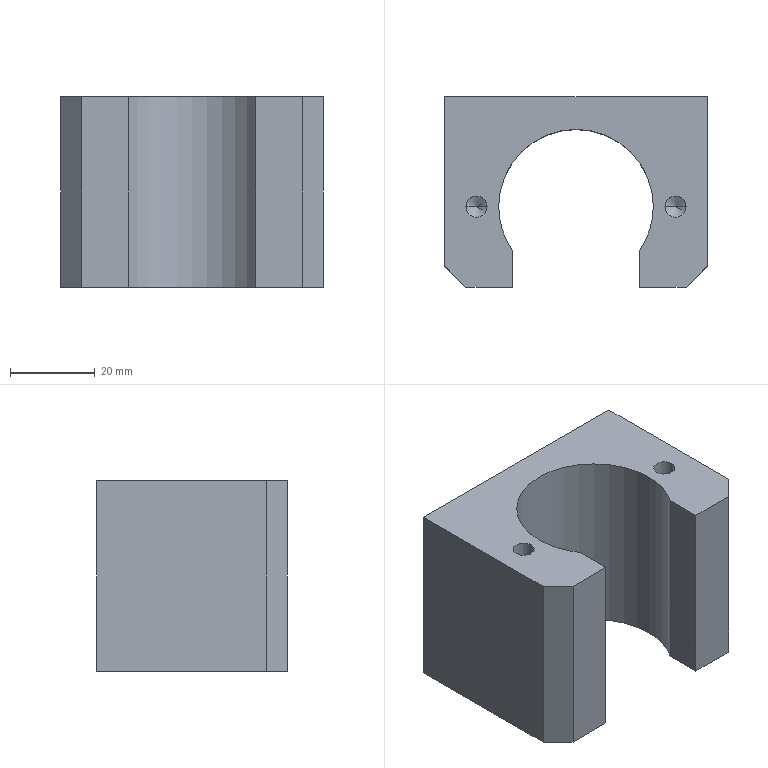Part | SolidWorks | features HoleWzd 2, Chamfer 1, Extrusion 1, ICE 1, MirrorPattern 1 | 1 solid | 46 faces | box 62 x 45 x 45 mm | volume 70731 mm3 | cylinder 19 | cone 16 | plane 11 | commonest cylinder face diameters 5 x16 36.5 x3
STEP:
#1=CARTESIAN_POINT('',(21.,-3.5,7.5));
#2=VERTEX_POINT('',#1);
#3=CARTESIAN_POINT('',(26.,-3.5,7.5));
#4=VERTEX_POINT('',#3);
#5=CARTESIAN_POINT('',(23.5,-3.5,7.5));
#6=DIRECTION('',(0.,0.,1.));
#7=DIRECTION('',(1.,0.,0.));
#8=AXIS2_PLACEMENT_3D('',#5,#6,#7);
#9=CIRCLE('',#8,2.5);
#10=EDGE_CURVE('',#2,#4,#9,.T.);
#11=ORIENTED_EDGE('',*,*,#10,.F.);
#12=CARTESIAN_POINT('',(21.,-3.5,22.5));
#13=VERTEX_POINT('',#12);
#14=CARTESIAN_POINT('',(21.,-3.5,22.5));
#15=DIRECTION('',(0.,0.,1.));
#16=VECTOR('',#15,1000.);
#17=LINE('',#14,#16);
#18=EDGE_CURVE('',#2,#13,#17,.T.);
#19=ORIENTED_EDGE('',*,*,#18,.T.);
#20=CARTESIAN_POINT('',(26.,-3.5,22.5));
#21=VERTEX_POINT('',#20);
#22=CARTESIAN_POINT('',(23.5,-3.5,22.5));
#23=DIRECTION('',(0.,0.,1.));
#24=DIRECTION('',(1.,0.,0.));
#25=AXIS2_PLACEMENT_3D('',#22,#23,#24);
#26=CIRCLE('',#25,2.5);
#27=EDGE_CURVE('',#13,#21,#26,.T.);
#28=ORIENTED_EDGE('',*,*,#27,.T.);
#29=CARTESIAN_POINT('',(26.,-3.5,22.5));
#30=DIRECTION('',(0.,0.,1.));
#31=VECTOR('',#30,1000.);
#32=LINE('',#29,#31);
#33=EDGE_CURVE('',#4,#21,#32,.T.);
#34=ORIENTED_EDGE('',*,*,#33,.F.);
#35=EDGE_LOOP('',(#11,#19,#28,#34));
#36=FACE_OUTER_BOUND('',#35,.T.);
#37=CARTESIAN_POINT('',(23.5,-3.5,22.5));
#38=DIRECTION('',(0.,0.,1.));
#39=DIRECTION('',(1.,0.,0.));
#40=AXIS2_PLACEMENT_3D('',#37,#38,#39);
#41=CYLINDRICAL_SURFACE('',#40,2.5);
#42=ADVANCED_FACE('',(#36),#41,.F.);
#43=CARTESIAN_POINT('',(23.5,-3.5,5.998));
#44=VERTEX_POINT('',#43);
#45=CARTESIAN_POINT('',(26.,-3.5,7.5));
#46=DIRECTION('',(0.8572,0.,0.515));
#47=VECTOR('',#46,1000.);
#48=LINE('',#45,#47);
#49=EDGE_CURVE('',#44,#4,#48,.T.);
#50=ORIENTED_EDGE('',*,*,#49,.F.);
#51=CARTESIAN_POINT('',(21.,-3.5,7.5));
#52=DIRECTION('',(-0.8572,0.,0.515));
#53=VECTOR('',#52,1000.);
#54=LINE('',#51,#53);
#55=EDGE_CURVE('',#44,#2,#54,.T.);
#56=ORIENTED_EDGE('',*,*,#55,.T.);
#57=ORIENTED_EDGE('',*,*,#10,.T.);
#58=EDGE_LOOP('',(#50,#56,#57));
#59=FACE_OUTER_BOUND('',#58,.T.);
#60=CARTESIAN_POINT('',(23.5,-3.5,7.5));
#61=DIRECTION('',(0.,0.,1.));
#62=DIRECTION('',(1.,0.,0.));
#63=AXIS2_PLACEMENT_3D('',#60,#61,#62);
#64=CONICAL_SURFACE('',#63,2.5,1.03);
#65=ADVANCED_FACE('',(#59),#64,.F.);
#66=CARTESIAN_POINT('',(-26.,-3.5,7.5));
#67=VERTEX_POINT('',#66);
#68=CARTESIAN_POINT('',(-21.,-3.5,7.5));
#69=VERTEX_POINT('',#68);
#70=CARTESIAN_POINT('',(-23.5,-3.5,7.5));
#71=DIRECTION('',(0.,0.,1.));
#72=DIRECTION('',(1.,0.,0.));
#73=AXIS2_PLACEMENT_3D('',#70,#71,#72);
#74=CIRCLE('',#73,2.5);
#75=EDGE_CURVE('',#67,#69,#74,.T.);
#76=ORIENTED_EDGE('',*,*,#75,.F.);
#77=CARTESIAN_POINT('',(-26.,-3.5,22.5));
#78=VERTEX_POINT('',#77);
#79=CARTESIAN_POINT('',(-26.,-3.5,22.5));
#80=DIRECTION('',(0.,0.,1.));
#81=VECTOR('',#80,1000.);
#82=LINE('',#79,#81);
#83=EDGE_CURVE('',#67,#78,#82,.T.);
#84=ORIENTED_EDGE('',*,*,#83,.T.);
#85=CARTESIAN_POINT('',(-21.,-3.5,22.5));
#86=VERTEX_POINT('',#85);
#87=CARTESIAN_POINT('',(-23.5,-3.5,22.5));
#88=DIRECTION('',(0.,0.,1.));
#89=DIRECTION('',(1.,0.,0.));
#90=AXIS2_PLACEMENT_3D('',#87,#88,#89);
#91=CIRCLE('',#90,2.5);
#92=EDGE_CURVE('',#78,#86,#91,.T.);
#93=ORIENTED_EDGE('',*,*,#92,.T.);
#94=CARTESIAN_POINT('',(-21.,-3.5,22.5));
#95=DIRECTION('',(0.,0.,1.));
#96=VECTOR('',#95,1000.);
#97=LINE('',#94,#96);
#98=EDGE_CURVE('',#69,#86,#97,.T.);
#99=ORIENTED_EDGE('',*,*,#98,.F.);
#100=EDGE_LOOP('',(#76,#84,#93,#99));
#101=FACE_OUTER_BOUND('',#100,.T.);
#102=CARTESIAN_POINT('',(-23.5,-3.5,22.5));
#103=DIRECTION('',(0.,0.,1.));
#104=DIRECTION('',(1.,0.,0.));
#105=AXIS2_PLACEMENT_3D('',#102,#103,#104);
#106=CYLINDRICAL_SURFACE('',#105,2.5);
#107=ADVANCED_FACE('',(#101),#106,.F.);
#108=CARTESIAN_POINT('',(-23.5,-3.5,5.998));
#109=VERTEX_POINT('',#108);
#110=CARTESIAN_POINT('',(-21.,-3.5,7.5));
#111=DIRECTION('',(0.8572,0.,0.515));
#112=VECTOR('',#111,1000.);
#113=LINE('',#110,#112);
#114=EDGE_CURVE('',#109,#69,#113,.T.);
#115=ORIENTED_EDGE('',*,*,#114,.F.);
#116=CARTESIAN_POINT('',(-26.,-3.5,7.5));
#117=DIRECTION('',(-0.8572,0.,0.515));
#118=VECTOR('',#117,1000.);
#119=LINE('',#116,#118);
#120=EDGE_CURVE('',#109,#67,#119,.T.);
#121=ORIENTED_EDGE('',*,*,#120,.T.);
#122=ORIENTED_EDGE('',*,*,#75,.T.);
#123=EDGE_LOOP('',(#115,#121,#122));
#124=FACE_OUTER_BOUND('',#123,.T.);
#125=CARTESIAN_POINT('',(-23.5,-3.5,7.5));
#126=DIRECTION('',(0.,0.,1.));
#127=DIRECTION('',(1.,0.,0.));
#128=AXIS2_PLACEMENT_3D('',#125,#126,#127);
#129=CONICAL_SURFACE('',#128,2.5,1.03);
#130=ADVANCED_FACE('',(#124),#129,.F.);
#131=CARTESIAN_POINT('',(26.,-3.5,-7.5));
#132=VERTEX_POINT('',#131);
#133=CARTESIAN_POINT('',(21.,-3.5,-7.5));
#134=VERTEX_POINT('',#133);
#135=CARTESIAN_POINT('',(23.5,-3.5,-7.5));
#136=DIRECTION('',(0.,0.,-1.));
#137=DIRECTION('',(-1.,0.,0.));
#138=AXIS2_PLACEMENT_3D('',#135,#136,#137);
#139=CIRCLE('',#138,2.5);
#140=EDGE_CURVE('',#132,#134,#139,.T.);
#141=ORIENTED_EDGE('',*,*,#140,.F.);
#142=CARTESIAN_POINT('',(26.,-3.5,-22.5));
#143=VERTEX_POINT('',#142);
#144=CARTESIAN_POINT('',(26.,-3.5,-22.5));
#145=DIRECTION('',(0.,0.,-1.));
#146=VECTOR('',#145,1000.);
#147=LINE('',#144,#146);
#148=EDGE_CURVE('',#132,#143,#147,.T.);
#149=ORIENTED_EDGE('',*,*,#148,.T.);
#150=CARTESIAN_POINT('',(21.,-3.5,-22.5));
#151=VERTEX_POINT('',#150);
#152=CARTESIAN_POINT('',(23.5,-3.5,-22.5));
#153=DIRECTION('',(0.,0.,-1.));
#154=DIRECTION('',(-1.,0.,0.));
#155=AXIS2_PLACEMENT_3D('',#152,#153,#154);
#156=CIRCLE('',#155,2.5);
#157=EDGE_CURVE('',#143,#151,#156,.T.);
#158=ORIENTED_EDGE('',*,*,#157,.T.);
#159=CARTESIAN_POINT('',(21.,-3.5,-22.5));
#160=DIRECTION('',(0.,0.,-1.));
#161=VECTOR('',#160,1000.);
#162=LINE('',#159,#161);
#163=EDGE_CURVE('',#134,#151,#162,.T.);
#164=ORIENTED_EDGE('',*,*,#163,.F.);
#165=EDGE_LOOP('',(#141,#149,#158,#164));
#166=FACE_OUTER_BOUND('',#165,.T.);
#167=CARTESIAN_POINT('',(23.5,-3.5,-22.5));
#168=DIRECTION('',(0.,0.,-1.));
#169=DIRECTION('',(-1.,0.,0.));
#170=AXIS2_PLACEMENT_3D('',#167,#168,#169);
#171=CYLINDRICAL_SURFACE('',#170,2.5);
#172=ADVANCED_FACE('',(#166),#171,.F.);
#173=CARTESIAN_POINT('',(23.5,-3.5,-5.998));
#174=VERTEX_POINT('',#173);
#175=CARTESIAN_POINT('',(21.,-3.5,-7.5));
#176=DIRECTION('',(-0.8572,0.,-0.515));
#177=VECTOR('',#176,1000.);
#178=LINE('',#175,#177);
#179=EDGE_CURVE('',#174,#134,#178,.T.);
#180=ORIENTED_EDGE('',*,*,#179,.F.);
#181=CARTESIAN_POINT('',(26.,-3.5,-7.5));
#182=DIRECTION('',(0.8572,0.,-0.515));
#183=VECTOR('',#182,1000.);
#184=LINE('',#181,#183);
#185=EDGE_CURVE('',#174,#132,#184,.T.);
#186=ORIENTED_EDGE('',*,*,#185,.T.);
#187=ORIENTED_EDGE('',*,*,#140,.T.);
#188=EDGE_LOOP('',(#180,#186,#187));
#189=FACE_OUTER_BOUND('',#188,.T.);
#190=CARTESIAN_POINT('',(23.5,-3.5,-7.5));
#191=DIRECTION('',(0.,0.,-1.));
#192=DIRECTION('',(-1.,0.,0.));
#193=AXIS2_PLACEMENT_3D('',#190,#191,#192);
#194=CONICAL_SURFACE('',#193,2.5,1.03);
#195=ADVANCED_FACE('',(#189),#194,.F.);
#196=CARTESIAN_POINT('',(-21.,-3.5,-7.5));
#197=VERTEX_POINT('',#196);
#198=CARTESIAN_POINT('',(-26.,-3.5,-7.5));
#199=VERTEX_POINT('',#198);
#200=CARTESIAN_POINT('',(-23.5,-3.5,-7.5));
#201=DIRECTION('',(0.,0.,-1.));
#202=DIRECTION('',(-1.,0.,0.));
#203=AXIS2_PLACEMENT_3D('',#200,#201,#202);
#204=CIRCLE('',#203,2.5);
#205=EDGE_CURVE('',#197,#199,#204,.T.);
#206=ORIENTED_EDGE('',*,*,#205,.F.);
#207=CARTESIAN_POINT('',(-21.,-3.5,-22.5));
#208=VERTEX_POINT('',#207);
#209=CARTESIAN_POINT('',(-21.,-3.5,-22.5));
#210=DIRECTION('',(0.,0.,-1.));
#211=VECTOR('',#210,1000.);
#212=LINE('',#209,#211);
#213=EDGE_CURVE('',#197,#208,#212,.T.);
#214=ORIENTED_EDGE('',*,*,#213,.T.);
#215=CARTESIAN_POINT('',(-26.,-3.5,-22.5));
#216=VERTEX_POINT('',#215);
#217=CARTESIAN_POINT('',(-23.5,-3.5,-22.5));
#218=DIRECTION('',(0.,0.,-1.));
#219=DIRECTION('',(-1.,0.,0.));
#220=AXIS2_PLACEMENT_3D('',#217,#218,#219);
#221=CIRCLE('',#220,2.5);
#222=EDGE_CURVE('',#208,#216,#221,.T.);
#223=ORIENTED_EDGE('',*,*,#222,.T.);
#224=CARTESIAN_POINT('',(-26.,-3.5,-22.5));
#225=DIRECTION('',(0.,0.,-1.));
#226=VECTOR('',#225,1000.);
#227=LINE('',#224,#226);
#228=EDGE_CURVE('',#199,#216,#227,.T.);
#229=ORIENTED_EDGE('',*,*,#228,.F.);
#230=EDGE_LOOP('',(#206,#214,#223,#229));
#231=FACE_OUTER_BOUND('',#230,.T.);
#232=CARTESIAN_POINT('',(-23.5,-3.5,-22.5));
#233=DIRECTION('',(0.,0.,-1.));
#234=DIRECTION('',(-1.,0.,0.));
#235=AXIS2_PLACEMENT_3D('',#232,#233,#234);
#236=CYLINDRICAL_SURFACE('',#235,2.5);
#237=ADVANCED_FACE('',(#231),#236,.F.);
#238=CARTESIAN_POINT('',(-23.5,-3.5,-5.998));
#239=VERTEX_POINT('',#238);
#240=CARTESIAN_POINT('',(-26.,-3.5,-7.5));
#241=DIRECTION('',(-0.8572,0.,-0.515));
#242=VECTOR('',#241,1000.);
#243=LINE('',#240,#242);
#244=EDGE_CURVE('',#239,#199,#243,.T.);
#245=ORIENTED_EDGE('',*,*,#244,.F.);
#246=CARTESIAN_POINT('',(-21.,-3.5,-7.5));
#247=DIRECTION('',(0.8572,0.,-0.515));
#248=VECTOR('',#247,1000.);
#249=LINE('',#246,#248);
#250=EDGE_CURVE('',#239,#197,#249,.T.);
#251=ORIENTED_EDGE('',*,*,#250,.T.);
#252=ORIENTED_EDGE('',*,*,#205,.T.);
#253=EDGE_LOOP('',(#245,#251,#252));
#254=FACE_OUTER_BOUND('',#253,.T.);
#255=CARTESIAN_POINT('',(-23.5,-3.5,-7.5));
#256=DIRECTION('',(0.,0.,-1.));
#257=DIRECTION('',(-1.,0.,0.));
#258=AXIS2_PLACEMENT_3D('',#255,#256,#257);
#259=CONICAL_SURFACE('',#258,2.5,1.03);
#260=ADVANCED_FACE('',(#254),#259,.F.);
#261=CARTESIAN_POINT('',(-25.,7.5,-17.5));
#262=VERTEX_POINT('',#261);
#263=CARTESIAN_POINT('',(-25.,7.5,-12.5));
#264=VERTEX_POINT('',#263);
#265=CARTESIAN_POINT('',(-25.,7.5,-15.));
#266=DIRECTION('',(0.,1.,0.));
#267=DIRECTION('',(0.,0.,1.));
#268=AXIS2_PLACEMENT_3D('',#265,#266,#267);
#269=CIRCLE('',#268,2.5);
#270=EDGE_CURVE('',#262,#264,#269,.T.);
#271=ORIENTED_EDGE('',*,*,#270,.F.);
#272=CARTESIAN_POINT('',(-25.,22.5,-17.5));
#273=VERTEX_POINT('',#272);
#274=CARTESIAN_POINT('',(-25.,22.5,-17.5));
#275=DIRECTION('',(0.,1.,0.));
#276=VECTOR('',#275,1000.);
#277=LINE('',#274,#276);
#278=EDGE_CURVE('',#262,#273,#277,.T.);
#279=ORIENTED_EDGE('',*,*,#278,.T.);
#280=CARTESIAN_POINT('',(-25.,22.5,-12.5));
#281=VERTEX_POINT('',#280);
#282=CARTESIAN_POINT('',(-25.,22.5,-15.));
#283=DIRECTION('',(0.,1.,0.));
#284=DIRECTION('',(0.,0.,1.));
#285=AXIS2_PLACEMENT_3D('',#282,#283,#284);
#286=CIRCLE('',#285,2.5);
#287=EDGE_CURVE('',#273,#281,#286,.T.);
#288=ORIENTED_EDGE('',*,*,#287,.T.);
#289=CARTESIAN_POINT('',(-25.,22.5,-12.5));
#290=DIRECTION('',(0.,1.,0.));
#291=VECTOR('',#290,1000.);
#292=LINE('',#289,#291);
#293=EDGE_CURVE('',#264,#281,#292,.T.);
#294=ORIENTED_EDGE('',*,*,#293,.F.);
#295=EDGE_LOOP('',(#271,#279,#288,#294));
#296=FACE_OUTER_BOUND('',#295,.T.);
#297=CARTESIAN_POINT('',(-25.,22.5,-15.));
#298=DIRECTION('',(0.,1.,0.));
#299=DIRECTION('',(0.,0.,1.));
#300=AXIS2_PLACEMENT_3D('',#297,#298,#299);
#301=CYLINDRICAL_SURFACE('',#300,2.5);
#302=ADVANCED_FACE('',(#296),#301,.F.);
#303=CARTESIAN_POINT('',(-25.,5.998,-15.));
#304=VERTEX_POINT('',#303);
#305=CARTESIAN_POINT('',(-25.,7.5,-12.5));
#306=DIRECTION('',(0.,0.515,0.8572));
#307=VECTOR('',#306,1000.);
#308=LINE('',#305,#307);
#309=EDGE_CURVE('',#304,#264,#308,.T.);
#310=ORIENTED_EDGE('',*,*,#309,.F.);
#311=CARTESIAN_POINT('',(-25.,7.5,-17.5));
#312=DIRECTION('',(0.,0.515,-0.8572));
#313=VECTOR('',#312,1000.);
#314=LINE('',#311,#313);
#315=EDGE_CURVE('',#304,#262,#314,.T.);
#316=ORIENTED_EDGE('',*,*,#315,.T.);
#317=ORIENTED_EDGE('',*,*,#270,.T.);
#318=EDGE_LOOP('',(#310,#316,#317));
#319=FACE_OUTER_BOUND('',#318,.T.);
#320=CARTESIAN_POINT('',(-25.,7.5,-15.));
#321=DIRECTION('',(0.,1.,0.));
#322=DIRECTION('',(0.,0.,1.));
#323=AXIS2_PLACEMENT_3D('',#320,#321,#322);
#324=CONICAL_SURFACE('',#323,2.5,1.03);
#325=ADVANCED_FACE('',(#319),#324,.F.);
#326=CARTESIAN_POINT('',(-25.,7.5,12.5));
#327=VERTEX_POINT('',#326);
#328=CARTESIAN_POINT('',(-25.,7.5,17.5));
#329=VERTEX_POINT('',#328);
#330=CARTESIAN_POINT('',(-25.,7.5,15.));
#331=DIRECTION('',(0.,1.,0.));
#332=DIRECTION('',(0.,0.,1.));
#333=AXIS2_PLACEMENT_3D('',#330,#331,#332);
#334=CIRCLE('',#333,2.5);
#335=EDGE_CURVE('',#327,#329,#334,.T.);
#336=ORIENTED_EDGE('',*,*,#335,.F.);
#337=CARTESIAN_POINT('',(-25.,22.5,12.5));
#338=VERTEX_POINT('',#337);
#339=CARTESIAN_POINT('',(-25.,22.5,12.5));
#340=DIRECTION('',(0.,1.,0.));
#341=VECTOR('',#340,1000.);
#342=LINE('',#339,#341);
#343=EDGE_CURVE('',#327,#338,#342,.T.);
#344=ORIENTED_EDGE('',*,*,#343,.T.);
#345=CARTESIAN_POINT('',(-25.,22.5,17.5));
#346=VERTEX_POINT('',#345);
#347=CARTESIAN_POINT('',(-25.,22.5,15.));
#348=DIRECTION('',(0.,1.,0.));
#349=DIRECTION('',(0.,0.,1.));
#350=AXIS2_PLACEMENT_3D('',#347,#348,#349);
#351=CIRCLE('',#350,2.5);
#352=EDGE_CURVE('',#338,#346,#351,.T.);
#353=ORIENTED_EDGE('',*,*,#352,.T.);
#354=CARTESIAN_POINT('',(-25.,22.5,17.5));
#355=DIRECTION('',(0.,1.,0.));
#356=VECTOR('',#355,1000.);
#357=LINE('',#354,#356);
#358=EDGE_CURVE('',#329,#346,#357,.T.);
#359=ORIENTED_EDGE('',*,*,#358,.F.);
#360=EDGE_LOOP('',(#336,#344,#353,#359));
#361=FACE_OUTER_BOUND('',#360,.T.);
#362=CARTESIAN_POINT('',(-25.,22.5,15.));
#363=DIRECTION('',(0.,1.,0.));
#364=DIRECTION('',(0.,0.,1.));
#365=AXIS2_PLACEMENT_3D('',#362,#363,#364);
#366=CYLINDRICAL_SURFACE('',#365,2.5);
#367=ADVANCED_FACE('',(#361),#366,.F.);
#368=CARTESIAN_POINT('',(-25.,5.998,15.));
#369=VERTEX_POINT('',#368);
#370=CARTESIAN_POINT('',(-25.,7.5,17.5));
#371=DIRECTION('',(0.,0.515,0.8572));
#372=VECTOR('',#371,1000.);
#373=LINE('',#370,#372);
#374=EDGE_CURVE('',#369,#329,#373,.T.);
#375=ORIENTED_EDGE('',*,*,#374,.F.);
#376=CARTESIAN_POINT('',(-25.,7.5,12.5));
#377=DIRECTION('',(0.,0.515,-0.8572));
#378=VECTOR('',#377,1000.);
#379=LINE('',#376,#378);
#380=EDGE_CURVE('',#369,#327,#379,.T.);
#381=ORIENTED_EDGE('',*,*,#380,.T.);
#382=ORIENTED_EDGE('',*,*,#335,.T.);
#383=EDGE_LOOP('',(#375,#381,#382));
#384=FACE_OUTER_BOUND('',#383,.T.);
#385=CARTESIAN_POINT('',(-25.,7.5,15.));
#386=DIRECTION('',(0.,1.,0.));
#387=DIRECTION('',(0.,0.,1.));
#388=AXIS2_PLACEMENT_3D('',#385,#386,#387);
#389=CONICAL_SURFACE('',#388,2.5,1.03);
#390=ADVANCED_FACE('',(#384),#389,.F.);
#391=CARTESIAN_POINT('',(25.,7.5,12.5));
#392=VERTEX_POINT('',#391);
#393=CARTESIAN_POINT('',(25.,7.5,17.5));
#394=VERTEX_POINT('',#393);
#395=CARTESIAN_POINT('',(25.,7.5,15.));
#396=DIRECTION('',(0.,1.,0.));
#397=DIRECTION('',(0.,0.,1.));
#398=AXIS2_PLACEMENT_3D('',#395,#396,#397);
#399=CIRCLE('',#398,2.5);
#400=EDGE_CURVE('',#392,#394,#399,.T.);
#401=ORIENTED_EDGE('',*,*,#400,.F.);
#402=CARTESIAN_POINT('',(25.,22.5,12.5));
#403=VERTEX_POINT('',#402);
#404=CARTESIAN_POINT('',(25.,22.5,12.5));
#405=DIRECTION('',(0.,1.,0.));
#406=VECTOR('',#405,1000.);
#407=LINE('',#404,#406);
#408=EDGE_CURVE('',#392,#403,#407,.T.);
#409=ORIENTED_EDGE('',*,*,#408,.T.);
#410=CARTESIAN_POINT('',(25.,22.5,17.5));
#411=VERTEX_POINT('',#410);
#412=CARTESIAN_POINT('',(25.,22.5,15.));
#413=DIRECTION('',(0.,1.,0.));
#414=DIRECTION('',(0.,0.,1.));
#415=AXIS2_PLACEMENT_3D('',#412,#413,#414);
#416=CIRCLE('',#415,2.5);
#417=EDGE_CURVE('',#403,#411,#416,.T.);
#418=ORIENTED_EDGE('',*,*,#417,.T.);
#419=CARTESIAN_POINT('',(25.,22.5,17.5));
#420=DIRECTION('',(0.,1.,0.));
#421=VECTOR('',#420,1000.);
#422=LINE('',#419,#421);
#423=EDGE_CURVE('',#394,#411,#422,.T.);
#424=ORIENTED_EDGE('',*,*,#423,.F.);
#425=EDGE_LOOP('',(#401,#409,#418,#424));
#426=FACE_OUTER_BOUND('',#425,.T.);
#427=CARTESIAN_POINT('',(25.,22.5,15.));
#428=DIRECTION('',(0.,1.,0.));
#429=DIRECTION('',(0.,0.,1.));
#430=AXIS2_PLACEMENT_3D('',#427,#428,#429);
#431=CYLINDRICAL_SURFACE('',#430,2.5);
#432=ADVANCED_FACE('',(#426),#431,.F.);
#433=CARTESIAN_POINT('',(25.,5.998,15.));
#434=VERTEX_POINT('',#433);
#435=CARTESIAN_POINT('',(25.,7.5,17.5));
#436=DIRECTION('',(0.,0.515,0.8572));
#437=VECTOR('',#436,1000.);
#438=LINE('',#435,#437);
#439=EDGE_CURVE('',#434,#394,#438,.T.);
#440=ORIENTED_EDGE('',*,*,#439,.F.);
#441=CARTESIAN_POINT('',(25.,7.5,12.5));
#442=DIRECTION('',(0.,0.515,-0.8572));
#443=VECTOR('',#442,1000.);
#444=LINE('',#441,#443);
#445=EDGE_CURVE('',#434,#392,#444,.T.);
#446=ORIENTED_EDGE('',*,*,#445,.T.);
#447=ORIENTED_EDGE('',*,*,#400,.T.);
#448=EDGE_LOOP('',(#440,#446,#447));
#449=FACE_OUTER_BOUND('',#448,.T.);
#450=CARTESIAN_POINT('',(25.,7.5,15.));
#451=DIRECTION('',(0.,1.,0.));
#452=DIRECTION('',(0.,0.,1.));
#453=AXIS2_PLACEMENT_3D('',#450,#451,#452);
#454=CONICAL_SURFACE('',#453,2.5,1.03);
#455=ADVANCED_FACE('',(#449),#454,.F.);
#456=CARTESIAN_POINT('',(25.,7.5,-17.5));
#457=VERTEX_POINT('',#456);
#458=CARTESIAN_POINT('',(25.,7.5,-12.5));
#459=VERTEX_POINT('',#458);
#460=CARTESIAN_POINT('',(25.,7.5,-15.));
#461=DIRECTION('',(0.,1.,0.));
#462=DIRECTION('',(0.,0.,1.));
#463=AXIS2_PLACEMENT_3D('',#460,#461,#462);
#464=CIRCLE('',#463,2.5);
#465=EDGE_CURVE('',#457,#459,#464,.T.);
#466=ORIENTED_EDGE('',*,*,#465,.F.);
#467=CARTESIAN_POINT('',(25.,22.5,-17.5));
#468=VERTEX_POINT('',#467);
#469=CARTESIAN_POINT('',(25.,22.5,-17.5));
#470=DIRECTION('',(0.,1.,0.));
#471=VECTOR('',#470,1000.);
#472=LINE('',#469,#471);
#473=EDGE_CURVE('',#457,#468,#472,.T.);
#474=ORIENTED_EDGE('',*,*,#473,.T.);
#475=CARTESIAN_POINT('',(25.,22.5,-12.5));
#476=VERTEX_POINT('',#475);
#477=CARTESIAN_POINT('',(25.,22.5,-15.));
#478=DIRECTION('',(0.,1.,0.));
#479=DIRECTION('',(0.,0.,1.));
#480=AXIS2_PLACEMENT_3D('',#477,#478,#479);
#481=CIRCLE('',#480,2.5);
#482=EDGE_CURVE('',#468,#476,#481,.T.);
#483=ORIENTED_EDGE('',*,*,#482,.T.);
#484=CARTESIAN_POINT('',(25.,22.5,-12.5));
#485=DIRECTION('',(0.,1.,0.));
#486=VECTOR('',#485,1000.);
#487=LINE('',#484,#486);
#488=EDGE_CURVE('',#459,#476,#487,.T.);
#489=ORIENTED_EDGE('',*,*,#488,.F.);
#490=EDGE_LOOP('',(#466,#474,#483,#489));
#491=FACE_OUTER_BOUND('',#490,.T.);
#492=CARTESIAN_POINT('',(25.,22.5,-15.));
#493=DIRECTION('',(0.,1.,0.));
#494=DIRECTION('',(0.,0.,1.));
#495=AXIS2_PLACEMENT_3D('',#492,#493,#494);
#496=CYLINDRICAL_SURFACE('',#495,2.5);
#497=ADVANCED_FACE('',(#491),#496,.F.);
#498=CARTESIAN_POINT('',(25.,5.998,-15.));
#499=VERTEX_POINT('',#498);
#500=CARTESIAN_POINT('',(25.,7.5,-12.5));
#501=DIRECTION('',(0.,0.515,0.8572));
#502=VECTOR('',#501,1000.);
#503=LINE('',#500,#502);
#504=EDGE_CURVE('',#499,#459,#503,.T.);
#505=ORIENTED_EDGE('',*,*,#504,.F.);
#506=CARTESIAN_POINT('',(25.,7.5,-17.5));
#507=DIRECTION('',(0.,0.515,-0.8572));
#508=VECTOR('',#507,1000.);
#509=LINE('',#506,#508);
#510=EDGE_CURVE('',#499,#457,#509,.T.);
#511=ORIENTED_EDGE('',*,*,#510,.T.);
#512=ORIENTED_EDGE('',*,*,#465,.T.);
#513=EDGE_LOOP('',(#505,#511,#512));
#514=FACE_OUTER_BOUND('',#513,.T.);
#515=CARTESIAN_POINT('',(25.,7.5,-15.));
#516=DIRECTION('',(0.,1.,0.));
#517=DIRECTION('',(0.,0.,1.));
#518=AXIS2_PLACEMENT_3D('',#515,#516,#517);
#519=CONICAL_SURFACE('',#518,2.5,1.03);
#520=ADVANCED_FACE('',(#514),#519,.F.);
#521=CARTESIAN_POINT('',(15.,-13.895,22.5));
#522=VERTEX_POINT('',#521);
#523=CARTESIAN_POINT('',(18.25,-3.5,22.5));
#524=VERTEX_POINT('',#523);
#525=CARTESIAN_POINT('',(0.,-3.5,22.5));
#526=DIRECTION('',(0.,0.,1.));
#527=DIRECTION('',(-1.,0.,0.));
#528=AXIS2_PLACEMENT_3D('',#525,#526,#527);
#529=CIRCLE('',#528,18.25);
#530=EDGE_CURVE('',#522,#524,#529,.T.);
#531=ORIENTED_EDGE('',*,*,#530,.T.);
#532=CARTESIAN_POINT('',(18.25,-3.5,-22.5));
#533=VERTEX_POINT('',#532);
#534=CARTESIAN_POINT('',(18.25,-3.5,74.652));
#535=DIRECTION('',(0.,0.,-1.));
#536=VECTOR('',#535,1000.);
#537=LINE('',#534,#536);
#538=EDGE_CURVE('',#524,#533,#537,.T.);
#539=ORIENTED_EDGE('',*,*,#538,.T.);
#540=CARTESIAN_POINT('',(15.,-13.895,-22.5));
#541=VERTEX_POINT('',#540);
#542=CARTESIAN_POINT('',(0.,-3.5,-22.5));
#543=DIRECTION('',(0.,0.,-1.));
#544=DIRECTION('',(-1.,0.,0.));
#545=AXIS2_PLACEMENT_3D('',#542,#543,#544);
#546=CIRCLE('',#545,18.25);
#547=EDGE_CURVE('',#533,#541,#546,.T.);
#548=ORIENTED_EDGE('',*,*,#547,.T.);
#549=CARTESIAN_POINT('',(15.,-13.895,74.652));
#550=DIRECTION('',(0.,0.,-1.));
#551=VECTOR('',#550,1000.);
#552=LINE('',#549,#551);
#553=EDGE_CURVE('',#522,#541,#552,.T.);
#554=ORIENTED_EDGE('',*,*,#553,.F.);
#555=EDGE_LOOP('',(#531,#539,#548,#554));
#556=FACE_OUTER_BOUND('',#555,.T.);
#557=CARTESIAN_POINT('',(0.,-3.5,74.652));
#558=DIRECTION('',(0.,0.,-1.));
#559=DIRECTION('',(-1.,0.,0.));
#560=AXIS2_PLACEMENT_3D('',#557,#558,#559);
#561=CYLINDRICAL_SURFACE('',#560,18.25);
#562=ADVANCED_FACE('',(#556),#561,.F.);
#563=ORIENTED_EDGE('',*,*,#538,.F.);
#564=CARTESIAN_POINT('',(-18.25,-3.5,22.5));
#565=VERTEX_POINT('',#564);
#566=CARTESIAN_POINT('',(0.,-3.5,22.5));
#567=DIRECTION('',(0.,0.,1.));
#568=DIRECTION('',(-1.,0.,0.));
#569=AXIS2_PLACEMENT_3D('',#566,#567,#568);
#570=CIRCLE('',#569,18.25);
#571=EDGE_CURVE('',#524,#565,#570,.T.);
#572=ORIENTED_EDGE('',*,*,#571,.T.);
#573=CARTESIAN_POINT('',(-18.25,-3.5,-22.5));
#574=VERTEX_POINT('',#573);
#575=CARTESIAN_POINT('',(-18.25,-3.5,74.652));
#576=DIRECTION('',(0.,0.,-1.));
#577=VECTOR('',#576,1000.);
#578=LINE('',#575,#577);
#579=EDGE_CURVE('',#565,#574,#578,.T.);
#580=ORIENTED_EDGE('',*,*,#579,.T.);
#581=CARTESIAN_POINT('',(0.,-3.5,-22.5));
#582=DIRECTION('',(0.,0.,-1.));
#583=DIRECTION('',(-1.,0.,0.));
#584=AXIS2_PLACEMENT_3D('',#581,#582,#583);
#585=CIRCLE('',#584,18.25);
#586=EDGE_CURVE('',#574,#533,#585,.T.);
#587=ORIENTED_EDGE('',*,*,#586,.T.);
#588=EDGE_LOOP('',(#563,#572,#580,#587));
#589=FACE_OUTER_BOUND('',#588,.T.);
#590=CARTESIAN_POINT('',(0.,-3.5,74.652));
#591=DIRECTION('',(0.,0.,-1.));
#592=DIRECTION('',(-1.,0.,0.));
#593=AXIS2_PLACEMENT_3D('',#590,#591,#592);
#594=CYLINDRICAL_SURFACE('',#593,18.25);
#595=ADVANCED_FACE('',(#589),#594,.F.);
#596=CARTESIAN_POINT('',(-26.,-22.5,22.5));
#597=VERTEX_POINT('',#596);
#598=CARTESIAN_POINT('',(-15.,-22.5,22.5));
#599=VERTEX_POINT('',#598);
#600=CARTESIAN_POINT('',(-31.,-22.5,22.5));
#601=DIRECTION('',(1.,0.,0.));
#602=VECTOR('',#601,1000.);
#603=LINE('',#600,#602);
#604=EDGE_CURVE('',#597,#599,#603,.T.);
#605=ORIENTED_EDGE('',*,*,#604,.F.);
#606=CARTESIAN_POINT('',(-26.,-22.5,-22.5));
#607=VERTEX_POINT('',#606);
#608=CARTESIAN_POINT('',(-26.,-22.5,-22.5));
#609=DIRECTION('',(0.,0.,-1.));
#610=VECTOR('',#609,1000.);
#611=LINE('',#608,#610);
#612=EDGE_CURVE('',#597,#607,#611,.T.);
#613=ORIENTED_EDGE('',*,*,#612,.T.);
#614=CARTESIAN_POINT('',(-15.,-22.5,-22.5));
#615=VERTEX_POINT('',#614);
#616=CARTESIAN_POINT('',(-31.,-22.5,-22.5));
#617=DIRECTION('',(-1.,0.,0.));
#618=VECTOR('',#617,1000.);
#619=LINE('',#616,#618);
#620=EDGE_CURVE('',#615,#607,#619,.T.);
#621=ORIENTED_EDGE('',*,*,#620,.F.);
#622=CARTESIAN_POINT('',(-15.,-22.5,74.652));
#623=DIRECTION('',(0.,0.,-1.));
#624=VECTOR('',#623,1000.);
#625=LINE('',#622,#624);
#626=EDGE_CURVE('',#599,#615,#625,.T.);
#627=ORIENTED_EDGE('',*,*,#626,.F.);
#628=EDGE_LOOP('',(#605,#613,#621,#627));
#629=FACE_OUTER_BOUND('',#628,.T.);
#630=CARTESIAN_POINT('',(0.,-22.5,0.));
#631=DIRECTION('',(0.,-1.,0.));
#632=DIRECTION('',(0.,0.,-1.));
#633=AXIS2_PLACEMENT_3D('',#630,#631,#632);
#634=PLANE('',#633);
#635=ADVANCED_FACE('',(#629),#634,.T.);
#636=CARTESIAN_POINT('',(31.,22.5,22.5));
#637=VERTEX_POINT('',#636);
#638=CARTESIAN_POINT('',(31.,-17.5,22.5));
#639=VERTEX_POINT('',#638);
#640=CARTESIAN_POINT('',(31.,22.5,22.5));
#641=DIRECTION('',(0.,-1.,0.));
#642=VECTOR('',#641,1000.);
#643=LINE('',#640,#642);
#644=EDGE_CURVE('',#637,#639,#643,.T.);
#645=ORIENTED_EDGE('',*,*,#644,.T.);
#646=CARTESIAN_POINT('',(31.,-17.5,-22.5));
#647=VERTEX_POINT('',#646);
#648=CARTESIAN_POINT('',(31.,-17.5,-22.5));
#649=DIRECTION('',(0.,0.,-1.));
#650=VECTOR('',#649,1000.);
#651=LINE('',#648,#650);
#652=EDGE_CURVE('',#639,#647,#651,.T.);
#653=ORIENTED_EDGE('',*,*,#652,.T.);
#654=CARTESIAN_POINT('',(31.,22.5,-22.5));
#655=VERTEX_POINT('',#654);
#656=CARTESIAN_POINT('',(31.,22.5,-22.5));
#657=DIRECTION('',(0.,-1.,0.));
#658=VECTOR('',#657,1000.);
#659=LINE('',#656,#658);
#660=EDGE_CURVE('',#655,#647,#659,.T.);
#661=ORIENTED_EDGE('',*,*,#660,.F.);
#662=CARTESIAN_POINT('',(31.,22.5,22.5));
#663=DIRECTION('',(0.,0.,-1.));
#664=VECTOR('',#663,1000.);
#665=LINE('',#662,#664);
#666=EDGE_CURVE('',#637,#655,#665,.T.);
#667=ORIENTED_EDGE('',*,*,#666,.F.);
#668=EDGE_LOOP('',(#645,#653,#661,#667));
#669=FACE_OUTER_BOUND('',#668,.T.);
#670=CARTESIAN_POINT('',(31.,22.5,22.5));
#671=DIRECTION('',(-1.,0.,0.));
#672=DIRECTION('',(0.,0.,1.));
#673=AXIS2_PLACEMENT_3D('',#670,#671,#672);
#674=PLANE('',#673);
#675=ADVANCED_FACE('',(#669),#674,.F.);
#676=CARTESIAN_POINT('',(23.5,-3.5,-22.5));
#677=DIRECTION('',(0.,0.,-1.));
#678=DIRECTION('',(-1.,0.,0.));
#679=AXIS2_PLACEMENT_3D('',#676,#677,#678);
#680=CIRCLE('',#679,2.5);
#681=EDGE_CURVE('',#151,#143,#680,.T.);
#682=ORIENTED_EDGE('',*,*,#681,.F.);
#683=ORIENTED_EDGE('',*,*,#157,.F.);
#684=EDGE_LOOP('',(#682,#683));
#685=FACE_BOUND('',#684,.T.);
#686=CARTESIAN_POINT('',(-23.5,-3.5,-22.5));
#687=DIRECTION('',(0.,0.,-1.));
#688=DIRECTION('',(-1.,0.,0.));
#689=AXIS2_PLACEMENT_3D('',#686,#687,#688);
#690=CIRCLE('',#689,2.5);
#691=EDGE_CURVE('',#216,#208,#690,.T.);
#692=ORIENTED_EDGE('',*,*,#691,.F.);
#693=ORIENTED_EDGE('',*,*,#222,.F.);
#694=EDGE_LOOP('',(#692,#693));
#695=FACE_BOUND('',#694,.T.);
#696=ORIENTED_EDGE('',*,*,#660,.T.);
#697=CARTESIAN_POINT('',(26.,-22.5,-22.5));
#698=VERTEX_POINT('',#697);
#699=CARTESIAN_POINT('',(31.,-17.5,-22.5));
#700=DIRECTION('',(-0.7071,-0.7071,0.));
#701=VECTOR('',#700,1000.);
#702=LINE('',#699,#701);
#703=EDGE_CURVE('',#647,#698,#702,.T.);
#704=ORIENTED_EDGE('',*,*,#703,.T.);
#705=CARTESIAN_POINT('',(15.,-22.5,-22.5));
#706=VERTEX_POINT('',#705);
#707=CARTESIAN_POINT('',(-31.,-22.5,-22.5));
#708=DIRECTION('',(-1.,0.,0.));
#709=VECTOR('',#708,1000.);
#710=LINE('',#707,#709);
#711=EDGE_CURVE('',#698,#706,#710,.T.);
#712=ORIENTED_EDGE('',*,*,#711,.T.);
#713=CARTESIAN_POINT('',(15.,-13.895,-22.5));
#714=DIRECTION('',(0.,-1.,0.));
#715=VECTOR('',#714,1000.);
#716=LINE('',#713,#715);
#717=EDGE_CURVE('',#541,#706,#716,.T.);
#718=ORIENTED_EDGE('',*,*,#717,.F.);
#719=ORIENTED_EDGE('',*,*,#547,.F.);
#720=ORIENTED_EDGE('',*,*,#586,.F.);
#721=CARTESIAN_POINT('',(-15.,-13.895,-22.5));
#722=VERTEX_POINT('',#721);
#723=CARTESIAN_POINT('',(0.,-3.5,-22.5));
#724=DIRECTION('',(0.,0.,-1.));
#725=DIRECTION('',(-1.,0.,0.));
#726=AXIS2_PLACEMENT_3D('',#723,#724,#725);
#727=CIRCLE('',#726,18.25);
#728=EDGE_CURVE('',#722,#574,#727,.T.);
#729=ORIENTED_EDGE('',*,*,#728,.F.);
#730=CARTESIAN_POINT('',(-15.,-13.895,-22.5));
#731=DIRECTION('',(0.,1.,0.));
#732=VECTOR('',#731,1000.);
#733=LINE('',#730,#732);
#734=EDGE_CURVE('',#615,#722,#733,.T.);
#735=ORIENTED_EDGE('',*,*,#734,.F.);
#736=ORIENTED_EDGE('',*,*,#620,.T.);
#737=CARTESIAN_POINT('',(-31.,-17.5,-22.5));
#738=VERTEX_POINT('',#737);
#739=CARTESIAN_POINT('',(-31.,-17.5,-22.5));
#740=DIRECTION('',(-0.7071,0.7071,0.));
#741=VECTOR('',#740,1000.);
#742=LINE('',#739,#741);
#743=EDGE_CURVE('',#607,#738,#742,.T.);
#744=ORIENTED_EDGE('',*,*,#743,.T.);
#745=CARTESIAN_POINT('',(-31.,22.5,-22.5));
#746=VERTEX_POINT('',#745);
#747=CARTESIAN_POINT('',(-31.,22.5,-22.5));
#748=DIRECTION('',(0.,-1.,0.));
#749=VECTOR('',#748,1000.);
#750=LINE('',#747,#749);
#751=EDGE_CURVE('',#746,#738,#750,.T.);
#752=ORIENTED_EDGE('',*,*,#751,.F.);
#753=CARTESIAN_POINT('',(-31.,22.5,-22.5));
#754=DIRECTION('',(-1.,0.,0.));
#755=VECTOR('',#754,1000.);
#756=LINE('',#753,#755);
#757=EDGE_CURVE('',#655,#746,#756,.T.);
#758=ORIENTED_EDGE('',*,*,#757,.F.);
#759=EDGE_LOOP('',(#696,#704,#712,#718,#719,#720,#729,#735,#736,#744,#752,#758));
#760=FACE_OUTER_BOUND('',#759,.T.);
#761=CARTESIAN_POINT('',(-31.,22.5,-22.5));
#762=DIRECTION('',(0.,0.,1.));
#763=DIRECTION('',(1.,0.,0.));
#764=AXIS2_PLACEMENT_3D('',#761,#762,#763);
#765=PLANE('',#764);
#766=ADVANCED_FACE('',(#685,#695,#760),#765,.F.);
#767=ORIENTED_EDGE('',*,*,#751,.T.);
#768=CARTESIAN_POINT('',(-31.,-17.5,22.5));
#769=VERTEX_POINT('',#768);
#770=CARTESIAN_POINT('',(-31.,-17.5,22.5));
#771=DIRECTION('',(0.,0.,1.));
#772=VECTOR('',#771,1000.);
#773=LINE('',#770,#772);
#774=EDGE_CURVE('',#738,#769,#773,.T.);
#775=ORIENTED_EDGE('',*,*,#774,.T.);
#776=CARTESIAN_POINT('',(-31.,22.5,22.5));
#777=VERTEX_POINT('',#776);
#778=CARTESIAN_POINT('',(-31.,22.5,22.5));
#779=DIRECTION('',(0.,-1.,0.));
#780=VECTOR('',#779,1000.);
#781=LINE('',#778,#780);
#782=EDGE_CURVE('',#777,#769,#781,.T.);
#783=ORIENTED_EDGE('',*,*,#782,.F.);
#784=CARTESIAN_POINT('',(-31.,22.5,22.5));
#785=DIRECTION('',(0.,0.,1.));
#786=VECTOR('',#785,1000.);
#787=LINE('',#784,#786);
#788=EDGE_CURVE('',#746,#777,#787,.T.);
#789=ORIENTED_EDGE('',*,*,#788,.F.);
#790=EDGE_LOOP('',(#767,#775,#783,#789));
#791=FACE_OUTER_BOUND('',#790,.T.);
#792=CARTESIAN_POINT('',(-31.,22.5,22.5));
#793=DIRECTION('',(1.,0.,0.));
#794=DIRECTION('',(0.,0.,-1.));
#795=AXIS2_PLACEMENT_3D('',#792,#793,#794);
#796=PLANE('',#795);
#797=ADVANCED_FACE('',(#791),#796,.F.);
#798=CARTESIAN_POINT('',(23.5,-3.5,22.5));
#799=DIRECTION('',(0.,0.,1.));
#800=DIRECTION('',(1.,0.,0.));
#801=AXIS2_PLACEMENT_3D('',#798,#799,#800);
#802=CIRCLE('',#801,2.5);
#803=EDGE_CURVE('',#21,#13,#802,.T.);
#804=ORIENTED_EDGE('',*,*,#803,.F.);
#805=ORIENTED_EDGE('',*,*,#27,.F.);
#806=EDGE_LOOP('',(#804,#805));
#807=FACE_BOUND('',#806,.T.);
#808=CARTESIAN_POINT('',(-23.5,-3.5,22.5));
#809=DIRECTION('',(0.,0.,1.));
#810=DIRECTION('',(1.,0.,0.));
#811=AXIS2_PLACEMENT_3D('',#808,#809,#810);
#812=CIRCLE('',#811,2.5);
#813=EDGE_CURVE('',#86,#78,#812,.T.);
#814=ORIENTED_EDGE('',*,*,#813,.F.);
#815=ORIENTED_EDGE('',*,*,#92,.F.);
#816=EDGE_LOOP('',(#814,#815));
#817=FACE_BOUND('',#816,.T.);
#818=CARTESIAN_POINT('',(15.,-22.5,22.5));
#819=VERTEX_POINT('',#818);
#820=CARTESIAN_POINT('',(26.,-22.5,22.5));
#821=VERTEX_POINT('',#820);
#822=CARTESIAN_POINT('',(-31.,-22.5,22.5));
#823=DIRECTION('',(1.,0.,0.));
#824=VECTOR('',#823,1000.);
#825=LINE('',#822,#824);
#826=EDGE_CURVE('',#819,#821,#825,.T.);
#827=ORIENTED_EDGE('',*,*,#826,.T.);
#828=CARTESIAN_POINT('',(31.,-17.5,22.5));
#829=DIRECTION('',(0.7071,0.7071,0.));
#830=VECTOR('',#829,1000.);
#831=LINE('',#828,#830);
#832=EDGE_CURVE('',#821,#639,#831,.T.);
#833=ORIENTED_EDGE('',*,*,#832,.T.);
#834=ORIENTED_EDGE('',*,*,#644,.F.);
#835=CARTESIAN_POINT('',(-31.,22.5,22.5));
#836=DIRECTION('',(1.,0.,0.));
#837=VECTOR('',#836,1000.);
#838=LINE('',#835,#837);
#839=EDGE_CURVE('',#777,#637,#838,.T.);
#840=ORIENTED_EDGE('',*,*,#839,.F.);
#841=ORIENTED_EDGE('',*,*,#782,.T.);
#842=CARTESIAN_POINT('',(-31.,-17.5,22.5));
#843=DIRECTION('',(0.7071,-0.7071,0.));
#844=VECTOR('',#843,1000.);
#845=LINE('',#842,#844);
#846=EDGE_CURVE('',#769,#597,#845,.T.);
#847=ORIENTED_EDGE('',*,*,#846,.T.);
#848=ORIENTED_EDGE('',*,*,#604,.T.);
#849=CARTESIAN_POINT('',(-15.,-13.895,22.5));
#850=VERTEX_POINT('',#849);
#851=CARTESIAN_POINT('',(-15.,-13.895,22.5));
#852=DIRECTION('',(0.,-1.,0.));
#853=VECTOR('',#852,1000.);
#854=LINE('',#851,#853);
#855=EDGE_CURVE('',#850,#599,#854,.T.);
#856=ORIENTED_EDGE('',*,*,#855,.F.);
#857=CARTESIAN_POINT('',(0.,-3.5,22.5));
#858=DIRECTION('',(0.,0.,1.));
#859=DIRECTION('',(-1.,0.,0.));
#860=AXIS2_PLACEMENT_3D('',#857,#858,#859);
#861=CIRCLE('',#860,18.25);
#862=EDGE_CURVE('',#565,#850,#861,.T.);
#863=ORIENTED_EDGE('',*,*,#862,.F.);
#864=ORIENTED_EDGE('',*,*,#571,.F.);
#865=ORIENTED_EDGE('',*,*,#530,.F.);
#866=CARTESIAN_POINT('',(15.,-13.895,22.5));
#867=DIRECTION('',(0.,1.,0.));
#868=VECTOR('',#867,1000.);
#869=LINE('',#866,#868);
#870=EDGE_CURVE('',#819,#522,#869,.T.);
#871=ORIENTED_EDGE('',*,*,#870,.F.);
#872=EDGE_LOOP('',(#827,#833,#834,#840,#841,#847,#848,#856,#863,#864,#865,#871));
#873=FACE_OUTER_BOUND('',#872,.T.);
#874=CARTESIAN_POINT('',(-31.,22.5,22.5));
#875=DIRECTION('',(0.,0.,-1.));
#876=DIRECTION('',(-1.,0.,0.));
#877=AXIS2_PLACEMENT_3D('',#874,#875,#876);
#878=PLANE('',#877);
#879=ADVANCED_FACE('',(#807,#817,#873),#878,.F.);
#880=CARTESIAN_POINT('',(-25.,22.5,-15.));
#881=DIRECTION('',(0.,1.,0.));
#882=DIRECTION('',(0.,0.,1.));
#883=AXIS2_PLACEMENT_3D('',#880,#881,#882);
#884=CIRCLE('',#883,2.5);
#885=EDGE_CURVE('',#281,#273,#884,.T.);
#886=ORIENTED_EDGE('',*,*,#885,.F.);
#887=ORIENTED_EDGE('',*,*,#287,.F.);
#888=EDGE_LOOP('',(#886,#887));
#889=FACE_BOUND('',#888,.T.);
#890=CARTESIAN_POINT('',(-25.,22.5,15.));
#891=DIRECTION('',(0.,1.,0.));
#892=DIRECTION('',(0.,0.,1.));
#893=AXIS2_PLACEMENT_3D('',#890,#891,#892);
#894=CIRCLE('',#893,2.5);
#895=EDGE_CURVE('',#346,#338,#894,.T.);
#896=ORIENTED_EDGE('',*,*,#895,.F.);
#897=ORIENTED_EDGE('',*,*,#352,.F.);
#898=EDGE_LOOP('',(#896,#897));
#899=FACE_BOUND('',#898,.T.);
#900=CARTESIAN_POINT('',(25.,22.5,15.));
#901=DIRECTION('',(0.,1.,0.));
#902=DIRECTION('',(0.,0.,1.));
#903=AXIS2_PLACEMENT_3D('',#900,#901,#902);
#904=CIRCLE('',#903,2.5);
#905=EDGE_CURVE('',#411,#403,#904,.T.);
#906=ORIENTED_EDGE('',*,*,#905,.F.);
#907=ORIENTED_EDGE('',*,*,#417,.F.);
#908=EDGE_LOOP('',(#906,#907));
#909=FACE_BOUND('',#908,.T.);
#910=CARTESIAN_POINT('',(25.,22.5,-15.));
#911=DIRECTION('',(0.,1.,0.));
#912=DIRECTION('',(0.,0.,1.));
#913=AXIS2_PLACEMENT_3D('',#910,#911,#912);
#914=CIRCLE('',#913,2.5);
#915=EDGE_CURVE('',#476,#468,#914,.T.);
#916=ORIENTED_EDGE('',*,*,#915,.F.);
#917=ORIENTED_EDGE('',*,*,#482,.F.);
#918=EDGE_LOOP('',(#916,#917));
#919=FACE_BOUND('',#918,.T.);
#920=ORIENTED_EDGE('',*,*,#666,.T.);
#921=ORIENTED_EDGE('',*,*,#757,.T.);
#922=ORIENTED_EDGE('',*,*,#788,.T.);
#923=ORIENTED_EDGE('',*,*,#839,.T.);
#924=EDGE_LOOP('',(#920,#921,#922,#923));
#925=FACE_OUTER_BOUND('',#924,.T.);
#926=CARTESIAN_POINT('',(0.,22.5,0.));
#927=DIRECTION('',(0.,-1.,0.));
#928=DIRECTION('',(0.,0.,-1.));
#929=AXIS2_PLACEMENT_3D('',#926,#927,#928);
#930=PLANE('',#929);
#931=ADVANCED_FACE('',(#889,#899,#909,#919,#925),#930,.F.);
#932=ORIENTED_EDGE('',*,*,#711,.F.);
#933=CARTESIAN_POINT('',(26.,-22.5,22.5));
#934=DIRECTION('',(0.,0.,1.));
#935=VECTOR('',#934,1000.);
#936=LINE('',#933,#935);
#937=EDGE_CURVE('',#698,#821,#936,.T.);
#938=ORIENTED_EDGE('',*,*,#937,.T.);
#939=ORIENTED_EDGE('',*,*,#826,.F.);
#940=CARTESIAN_POINT('',(15.,-22.5,74.652));
#941=DIRECTION('',(0.,0.,-1.));
#942=VECTOR('',#941,1000.);
#943=LINE('',#940,#942);
#944=EDGE_CURVE('',#819,#706,#943,.T.);
#945=ORIENTED_EDGE('',*,*,#944,.T.);
#946=EDGE_LOOP('',(#932,#938,#939,#945));
#947=FACE_OUTER_BOUND('',#946,.T.);
#948=CARTESIAN_POINT('',(0.,-22.5,0.));
#949=DIRECTION('',(0.,-1.,0.));
#950=DIRECTION('',(0.,0.,-1.));
#951=AXIS2_PLACEMENT_3D('',#948,#949,#950);
#952=PLANE('',#951);
#953=ADVANCED_FACE('',(#947),#952,.T.);
#954=ORIENTED_EDGE('',*,*,#579,.F.);
#955=ORIENTED_EDGE('',*,*,#862,.T.);
#956=CARTESIAN_POINT('',(-15.,-13.895,74.652));
#957=DIRECTION('',(0.,0.,-1.));
#958=VECTOR('',#957,1000.);
#959=LINE('',#956,#958);
#960=EDGE_CURVE('',#850,#722,#959,.T.);
#961=ORIENTED_EDGE('',*,*,#960,.T.);
#962=ORIENTED_EDGE('',*,*,#728,.T.);
#963=EDGE_LOOP('',(#954,#955,#961,#962));
#964=FACE_OUTER_BOUND('',#963,.T.);
#965=CARTESIAN_POINT('',(0.,-3.5,74.652));
#966=DIRECTION('',(0.,0.,-1.));
#967=DIRECTION('',(-1.,0.,0.));
#968=AXIS2_PLACEMENT_3D('',#965,#966,#967);
#969=CYLINDRICAL_SURFACE('',#968,18.25);
#970=ADVANCED_FACE('',(#964),#969,.F.);
#971=ORIENTED_EDGE('',*,*,#855,.T.);
#972=ORIENTED_EDGE('',*,*,#626,.T.);
#973=ORIENTED_EDGE('',*,*,#734,.T.);
#974=ORIENTED_EDGE('',*,*,#960,.F.);
#975=EDGE_LOOP('',(#971,#972,#973,#974));
#976=FACE_OUTER_BOUND('',#975,.T.);
#977=CARTESIAN_POINT('',(-15.,-13.895,74.652));
#978=DIRECTION('',(-1.,0.,0.));
#979=DIRECTION('',(0.,-1.,0.));
#980=AXIS2_PLACEMENT_3D('',#977,#978,#979);
#981=PLANE('',#980);
#982=ADVANCED_FACE('',(#976),#981,.F.);
#983=ORIENTED_EDGE('',*,*,#870,.T.);
#984=ORIENTED_EDGE('',*,*,#553,.T.);
#985=ORIENTED_EDGE('',*,*,#717,.T.);
#986=ORIENTED_EDGE('',*,*,#944,.F.);
#987=EDGE_LOOP('',(#983,#984,#985,#986));
#988=FACE_OUTER_BOUND('',#987,.T.);
#989=CARTESIAN_POINT('',(15.,-13.895,74.652));
#990=DIRECTION('',(1.,0.,0.));
#991=DIRECTION('',(0.,0.,-1.));
#992=AXIS2_PLACEMENT_3D('',#989,#990,#991);
#993=PLANE('',#992);
#994=ADVANCED_FACE('',(#988),#993,.F.);
#995=ORIENTED_EDGE('',*,*,#832,.F.);
#996=ORIENTED_EDGE('',*,*,#937,.F.);
#997=ORIENTED_EDGE('',*,*,#703,.F.);
#998=ORIENTED_EDGE('',*,*,#652,.F.);
#999=EDGE_LOOP('',(#995,#996,#997,#998));
#1000=FACE_OUTER_BOUND('',#999,.T.);
#1001=CARTESIAN_POINT('',(31.,-17.5,22.5));
#1002=DIRECTION('',(0.7071,-0.7071,0.));
#1003=DIRECTION('',(0.,0.,1.));
#1004=AXIS2_PLACEMENT_3D('',#1001,#1002,#1003);
#1005=PLANE('',#1004);
#1006=ADVANCED_FACE('',(#1000),#1005,.T.);
#1007=ORIENTED_EDGE('',*,*,#743,.F.);
#1008=ORIENTED_EDGE('',*,*,#612,.F.);
#1009=ORIENTED_EDGE('',*,*,#846,.F.);
#1010=ORIENTED_EDGE('',*,*,#774,.F.);
#1011=EDGE_LOOP('',(#1007,#1008,#1009,#1010));
#1012=FACE_OUTER_BOUND('',#1011,.T.);
#1013=CARTESIAN_POINT('',(-31.,-17.5,22.5));
#1014=DIRECTION('',(-0.7071,-0.7071,0.));
#1015=DIRECTION('',(0.,0.,-1.));
#1016=AXIS2_PLACEMENT_3D('',#1013,#1014,#1015);
#1017=PLANE('',#1016);
#1018=ADVANCED_FACE('',(#1012),#1017,.T.);
#1019=ORIENTED_EDGE('',*,*,#510,.F.);
#1020=ORIENTED_EDGE('',*,*,#504,.T.);
#1021=CARTESIAN_POINT('',(25.,7.5,-15.));
#1022=DIRECTION('',(0.,1.,0.));
#1023=DIRECTION('',(0.,0.,1.));
#1024=AXIS2_PLACEMENT_3D('',#1021,#1022,#1023);
#1025=CIRCLE('',#1024,2.5);
#1026=EDGE_CURVE('',#459,#457,#1025,.T.);
#1027=ORIENTED_EDGE('',*,*,#1026,.T.);
#1028=EDGE_LOOP('',(#1019,#1020,#1027));
#1029=FACE_OUTER_BOUND('',#1028,.T.);
#1030=CARTESIAN_POINT('',(25.,7.5,-15.));
#1031=DIRECTION('',(0.,1.,0.));
#1032=DIRECTION('',(0.,0.,1.));
#1033=AXIS2_PLACEMENT_3D('',#1030,#1031,#1032);
#1034=CONICAL_SURFACE('',#1033,2.5,1.03);
#1035=ADVANCED_FACE('',(#1029),#1034,.F.);
#1036=ORIENTED_EDGE('',*,*,#473,.F.);
#1037=ORIENTED_EDGE('',*,*,#1026,.F.);
#1038=ORIENTED_EDGE('',*,*,#488,.T.);
#1039=ORIENTED_EDGE('',*,*,#915,.T.);
#1040=EDGE_LOOP('',(#1036,#1037,#1038,#1039));
#1041=FACE_OUTER_BOUND('',#1040,.T.);
#1042=CARTESIAN_POINT('',(25.,22.5,-15.));
#1043=DIRECTION('',(0.,1.,0.));
#1044=DIRECTION('',(0.,0.,1.));
#1045=AXIS2_PLACEMENT_3D('',#1042,#1043,#1044);
#1046=CYLINDRICAL_SURFACE('',#1045,2.5);
#1047=ADVANCED_FACE('',(#1041),#1046,.F.);
#1048=ORIENTED_EDGE('',*,*,#445,.F.);
#1049=ORIENTED_EDGE('',*,*,#439,.T.);
#1050=CARTESIAN_POINT('',(25.,7.5,15.));
#1051=DIRECTION('',(0.,1.,0.));
#1052=DIRECTION('',(0.,0.,1.));
#1053=AXIS2_PLACEMENT_3D('',#1050,#1051,#1052);
#1054=CIRCLE('',#1053,2.5);
#1055=EDGE_CURVE('',#394,#392,#1054,.T.);
#1056=ORIENTED_EDGE('',*,*,#1055,.T.);
#1057=EDGE_LOOP('',(#1048,#1049,#1056));
#1058=FACE_OUTER_BOUND('',#1057,.T.);
#1059=CARTESIAN_POINT('',(25.,7.5,15.));
#1060=DIRECTION('',(0.,1.,0.));
#1061=DIRECTION('',(0.,0.,1.));
#1062=AXIS2_PLACEMENT_3D('',#1059,#1060,#1061);
#1063=CONICAL_SURFACE('',#1062,2.5,1.03);
#1064=ADVANCED_FACE('',(#1058),#1063,.F.);
#1065=ORIENTED_EDGE('',*,*,#408,.F.);
#1066=ORIENTED_EDGE('',*,*,#1055,.F.);
#1067=ORIENTED_EDGE('',*,*,#423,.T.);
#1068=ORIENTED_EDGE('',*,*,#905,.T.);
#1069=EDGE_LOOP('',(#1065,#1066,#1067,#1068));
#1070=FACE_OUTER_BOUND('',#1069,.T.);
#1071=CARTESIAN_POINT('',(25.,22.5,15.));
#1072=DIRECTION('',(0.,1.,0.));
#1073=DIRECTION('',(0.,0.,1.));
#1074=AXIS2_PLACEMENT_3D('',#1071,#1072,#1073);
#1075=CYLINDRICAL_SURFACE('',#1074,2.5);
#1076=ADVANCED_FACE('',(#1070),#1075,.F.);
#1077=ORIENTED_EDGE('',*,*,#380,.F.);
#1078=ORIENTED_EDGE('',*,*,#374,.T.);
#1079=CARTESIAN_POINT('',(-25.,7.5,15.));
#1080=DIRECTION('',(0.,1.,0.));
#1081=DIRECTION('',(0.,0.,1.));
#1082=AXIS2_PLACEMENT_3D('',#1079,#1080,#1081);
#1083=CIRCLE('',#1082,2.5);
#1084=EDGE_CURVE('',#329,#327,#1083,.T.);
#1085=ORIENTED_EDGE('',*,*,#1084,.T.);
#1086=EDGE_LOOP('',(#1077,#1078,#1085));
#1087=FACE_OUTER_BOUND('',#1086,.T.);
#1088=CARTESIAN_POINT('',(-25.,7.5,15.));
#1089=DIRECTION('',(0.,1.,0.));
#1090=DIRECTION('',(0.,0.,1.));
#1091=AXIS2_PLACEMENT_3D('',#1088,#1089,#1090);
#1092=CONICAL_SURFACE('',#1091,2.5,1.03);
#1093=ADVANCED_FACE('',(#1087),#1092,.F.);
#1094=ORIENTED_EDGE('',*,*,#343,.F.);
#1095=ORIENTED_EDGE('',*,*,#1084,.F.);
#1096=ORIENTED_EDGE('',*,*,#358,.T.);
#1097=ORIENTED_EDGE('',*,*,#895,.T.);
#1098=EDGE_LOOP('',(#1094,#1095,#1096,#1097));
#1099=FACE_OUTER_BOUND('',#1098,.T.);
#1100=CARTESIAN_POINT('',(-25.,22.5,15.));
#1101=DIRECTION('',(0.,1.,0.));
#1102=DIRECTION('',(0.,0.,1.));
#1103=AXIS2_PLACEMENT_3D('',#1100,#1101,#1102);
#1104=CYLINDRICAL_SURFACE('',#1103,2.5);
#1105=ADVANCED_FACE('',(#1099),#1104,.F.);
#1106=ORIENTED_EDGE('',*,*,#315,.F.);
#1107=ORIENTED_EDGE('',*,*,#309,.T.);
#1108=CARTESIAN_POINT('',(-25.,7.5,-15.));
#1109=DIRECTION('',(0.,1.,0.));
#1110=DIRECTION('',(0.,0.,1.));
#1111=AXIS2_PLACEMENT_3D('',#1108,#1109,#1110);
#1112=CIRCLE('',#1111,2.5);
#1113=EDGE_CURVE('',#264,#262,#1112,.T.);
#1114=ORIENTED_EDGE('',*,*,#1113,.T.);
#1115=EDGE_LOOP('',(#1106,#1107,#1114));
#1116=FACE_OUTER_BOUND('',#1115,.T.);
#1117=CARTESIAN_POINT('',(-25.,7.5,-15.));
#1118=DIRECTION('',(0.,1.,0.));
#1119=DIRECTION('',(0.,0.,1.));
#1120=AXIS2_PLACEMENT_3D('',#1117,#1118,#1119);
#1121=CONICAL_SURFACE('',#1120,2.5,1.03);
#1122=ADVANCED_FACE('',(#1116),#1121,.F.);
#1123=ORIENTED_EDGE('',*,*,#278,.F.);
#1124=ORIENTED_EDGE('',*,*,#1113,.F.);
#1125=ORIENTED_EDGE('',*,*,#293,.T.);
#1126=ORIENTED_EDGE('',*,*,#885,.T.);
#1127=EDGE_LOOP('',(#1123,#1124,#1125,#1126));
#1128=FACE_OUTER_BOUND('',#1127,.T.);
#1129=CARTESIAN_POINT('',(-25.,22.5,-15.));
#1130=DIRECTION('',(0.,1.,0.));
#1131=DIRECTION('',(0.,0.,1.));
#1132=AXIS2_PLACEMENT_3D('',#1129,#1130,#1131);
#1133=CYLINDRICAL_SURFACE('',#1132,2.5);
#1134=ADVANCED_FACE('',(#1128),#1133,.F.);
#1135=ORIENTED_EDGE('',*,*,#250,.F.);
#1136=ORIENTED_EDGE('',*,*,#244,.T.);
#1137=CARTESIAN_POINT('',(-23.5,-3.5,-7.5));
#1138=DIRECTION('',(0.,0.,-1.));
#1139=DIRECTION('',(-1.,0.,0.));
#1140=AXIS2_PLACEMENT_3D('',#1137,#1138,#1139);
#1141=CIRCLE('',#1140,2.5);
#1142=EDGE_CURVE('',#199,#197,#1141,.T.);
#1143=ORIENTED_EDGE('',*,*,#1142,.T.);
#1144=EDGE_LOOP('',(#1135,#1136,#1143));
#1145=FACE_OUTER_BOUND('',#1144,.T.);
#1146=CARTESIAN_POINT('',(-23.5,-3.5,-7.5));
#1147=DIRECTION('',(0.,0.,-1.));
#1148=DIRECTION('',(-1.,0.,0.));
#1149=AXIS2_PLACEMENT_3D('',#1146,#1147,#1148);
#1150=CONICAL_SURFACE('',#1149,2.5,1.03);
#1151=ADVANCED_FACE('',(#1145),#1150,.F.);
#1152=ORIENTED_EDGE('',*,*,#213,.F.);
#1153=ORIENTED_EDGE('',*,*,#1142,.F.);
#1154=ORIENTED_EDGE('',*,*,#228,.T.);
#1155=ORIENTED_EDGE('',*,*,#691,.T.);
#1156=EDGE_LOOP('',(#1152,#1153,#1154,#1155));
#1157=FACE_OUTER_BOUND('',#1156,.T.);
#1158=CARTESIAN_POINT('',(-23.5,-3.5,-22.5));
#1159=DIRECTION('',(0.,0.,-1.));
#1160=DIRECTION('',(-1.,0.,0.));
#1161=AXIS2_PLACEMENT_3D('',#1158,#1159,#1160);
#1162=CYLINDRICAL_SURFACE('',#1161,2.5);
#1163=ADVANCED_FACE('',(#1157),#1162,.F.);
#1164=ORIENTED_EDGE('',*,*,#185,.F.);
#1165=ORIENTED_EDGE('',*,*,#179,.T.);
#1166=CARTESIAN_POINT('',(23.5,-3.5,-7.5));
#1167=DIRECTION('',(0.,0.,-1.));
#1168=DIRECTION('',(-1.,0.,0.));
#1169=AXIS2_PLACEMENT_3D('',#1166,#1167,#1168);
#1170=CIRCLE('',#1169,2.5);
#1171=EDGE_CURVE('',#134,#132,#1170,.T.);
#1172=ORIENTED_EDGE('',*,*,#1171,.T.);
#1173=EDGE_LOOP('',(#1164,#1165,#1172));
#1174=FACE_OUTER_BOUND('',#1173,.T.);
#1175=CARTESIAN_POINT('',(23.5,-3.5,-7.5));
#1176=DIRECTION('',(0.,0.,-1.));
#1177=DIRECTION('',(-1.,0.,0.));
#1178=AXIS2_PLACEMENT_3D('',#1175,#1176,#1177);
#1179=CONICAL_SURFACE('',#1178,2.5,1.03);
#1180=ADVANCED_FACE('',(#1174),#1179,.F.);
#1181=ORIENTED_EDGE('',*,*,#148,.F.);
#1182=ORIENTED_EDGE('',*,*,#1171,.F.);
#1183=ORIENTED_EDGE('',*,*,#163,.T.);
#1184=ORIENTED_EDGE('',*,*,#681,.T.);
#1185=EDGE_LOOP('',(#1181,#1182,#1183,#1184));
#1186=FACE_OUTER_BOUND('',#1185,.T.);
#1187=CARTESIAN_POINT('',(23.5,-3.5,-22.5));
#1188=DIRECTION('',(0.,0.,-1.));
#1189=DIRECTION('',(-1.,0.,0.));
#1190=AXIS2_PLACEMENT_3D('',#1187,#1188,#1189);
#1191=CYLINDRICAL_SURFACE('',#1190,2.5);
#1192=ADVANCED_FACE('',(#1186),#1191,.F.);
#1193=ORIENTED_EDGE('',*,*,#120,.F.);
#1194=ORIENTED_EDGE('',*,*,#114,.T.);
#1195=CARTESIAN_POINT('',(-23.5,-3.5,7.5));
#1196=DIRECTION('',(0.,0.,1.));
#1197=DIRECTION('',(1.,0.,0.));
#1198=AXIS2_PLACEMENT_3D('',#1195,#1196,#1197);
#1199=CIRCLE('',#1198,2.5);
#1200=EDGE_CURVE('',#69,#67,#1199,.T.);
#1201=ORIENTED_EDGE('',*,*,#1200,.T.);
#1202=EDGE_LOOP('',(#1193,#1194,#1201));
#1203=FACE_OUTER_BOUND('',#1202,.T.);
#1204=CARTESIAN_POINT('',(-23.5,-3.5,7.5));
#1205=DIRECTION('',(0.,0.,1.));
#1206=DIRECTION('',(1.,0.,0.));
#1207=AXIS2_PLACEMENT_3D('',#1204,#1205,#1206);
#1208=CONICAL_SURFACE('',#1207,2.5,1.03);
#1209=ADVANCED_FACE('',(#1203),#1208,.F.);
#1210=ORIENTED_EDGE('',*,*,#83,.F.);
#1211=ORIENTED_EDGE('',*,*,#1200,.F.);
#1212=ORIENTED_EDGE('',*,*,#98,.T.);
#1213=ORIENTED_EDGE('',*,*,#813,.T.);
#1214=EDGE_LOOP('',(#1210,#1211,#1212,#1213));
#1215=FACE_OUTER_BOUND('',#1214,.T.);
#1216=CARTESIAN_POINT('',(-23.5,-3.5,22.5));
#1217=DIRECTION('',(0.,0.,1.));
#1218=DIRECTION('',(1.,0.,0.));
#1219=AXIS2_PLACEMENT_3D('',#1216,#1217,#1218);
#1220=CYLINDRICAL_SURFACE('',#1219,2.5);
#1221=ADVANCED_FACE('',(#1215),#1220,.F.);
#1222=ORIENTED_EDGE('',*,*,#55,.F.);
#1223=ORIENTED_EDGE('',*,*,#49,.T.);
#1224=CARTESIAN_POINT('',(23.5,-3.5,7.5));
#1225=DIRECTION('',(0.,0.,1.));
#1226=DIRECTION('',(1.,0.,0.));
#1227=AXIS2_PLACEMENT_3D('',#1224,#1225,#1226);
#1228=CIRCLE('',#1227,2.5);
#1229=EDGE_CURVE('',#4,#2,#1228,.T.);
#1230=ORIENTED_EDGE('',*,*,#1229,.T.);
#1231=EDGE_LOOP('',(#1222,#1223,#1230));
#1232=FACE_OUTER_BOUND('',#1231,.T.);
#1233=CARTESIAN_POINT('',(23.5,-3.5,7.5));
#1234=DIRECTION('',(0.,0.,1.));
#1235=DIRECTION('',(1.,0.,0.));
#1236=AXIS2_PLACEMENT_3D('',#1233,#1234,#1235);
#1237=CONICAL_SURFACE('',#1236,2.5,1.03);
#1238=ADVANCED_FACE('',(#1232),#1237,.F.);
#1239=ORIENTED_EDGE('',*,*,#18,.F.);
#1240=ORIENTED_EDGE('',*,*,#1229,.F.);
#1241=ORIENTED_EDGE('',*,*,#33,.T.);
#1242=ORIENTED_EDGE('',*,*,#803,.T.);
#1243=EDGE_LOOP('',(#1239,#1240,#1241,#1242));
#1244=FACE_OUTER_BOUND('',#1243,.T.);
#1245=CARTESIAN_POINT('',(23.5,-3.5,22.5));
#1246=DIRECTION('',(0.,0.,1.));
#1247=DIRECTION('',(1.,0.,0.));
#1248=AXIS2_PLACEMENT_3D('',#1245,#1246,#1247);
#1249=CYLINDRICAL_SURFACE('',#1248,2.5);
#1250=ADVANCED_FACE('',(#1244),#1249,.F.);
#1251=CLOSED_SHELL('',(#42,#65,#107,#130,#172,#195,#237,#260,#302,#325,#367,#390,#432,#455,#497,#520,#562,#595,#635,#675,#766,#797,#879,#931,#953,#970,#982,#994,#1006,#1018,#1035,#1047,#1064,#1076,#1093,#1105,#1122,#1134,#1151,#1163,#1180,#1192,#1209,#1221,#1238,#1250));
#1252=MANIFOLD_SOLID_BREP('',#1251);
#1253=CARTESIAN_POINT('',(0.,0.,0.));
#1254=DIRECTION('',(0.,0.,1.));
#1255=DIRECTION('',(1.,0.,0.));
#1256=AXIS2_PLACEMENT_3D('',#1253,#1254,#1255);
#1257=(LENGTH_UNIT()NAMED_UNIT(*)SI_UNIT(.MILLI.,.METRE.));
#1258=UNCERTAINTY_MEASURE_WITH_UNIT(LENGTH_MEASURE(0.00001),#1257,'','');
#1259=(NAMED_UNIT(*)PLANE_ANGLE_UNIT()SI_UNIT($,.RADIAN.));
#1260=(NAMED_UNIT(*)SI_UNIT($,.STERADIAN.)SOLID_ANGLE_UNIT());
#1261=(GEOMETRIC_REPRESENTATION_CONTEXT(3)GLOBAL_UNCERTAINTY_ASSIGNED_CONTEXT((#1258))GLOBAL_UNIT_ASSIGNED_CONTEXT((#1257,#1259,#1260))REPRESENTATION_CONTEXT('',''));
#1262=ADVANCED_BREP_SHAPE_REPRESENTATION('',(#1252,#1256),#1261);